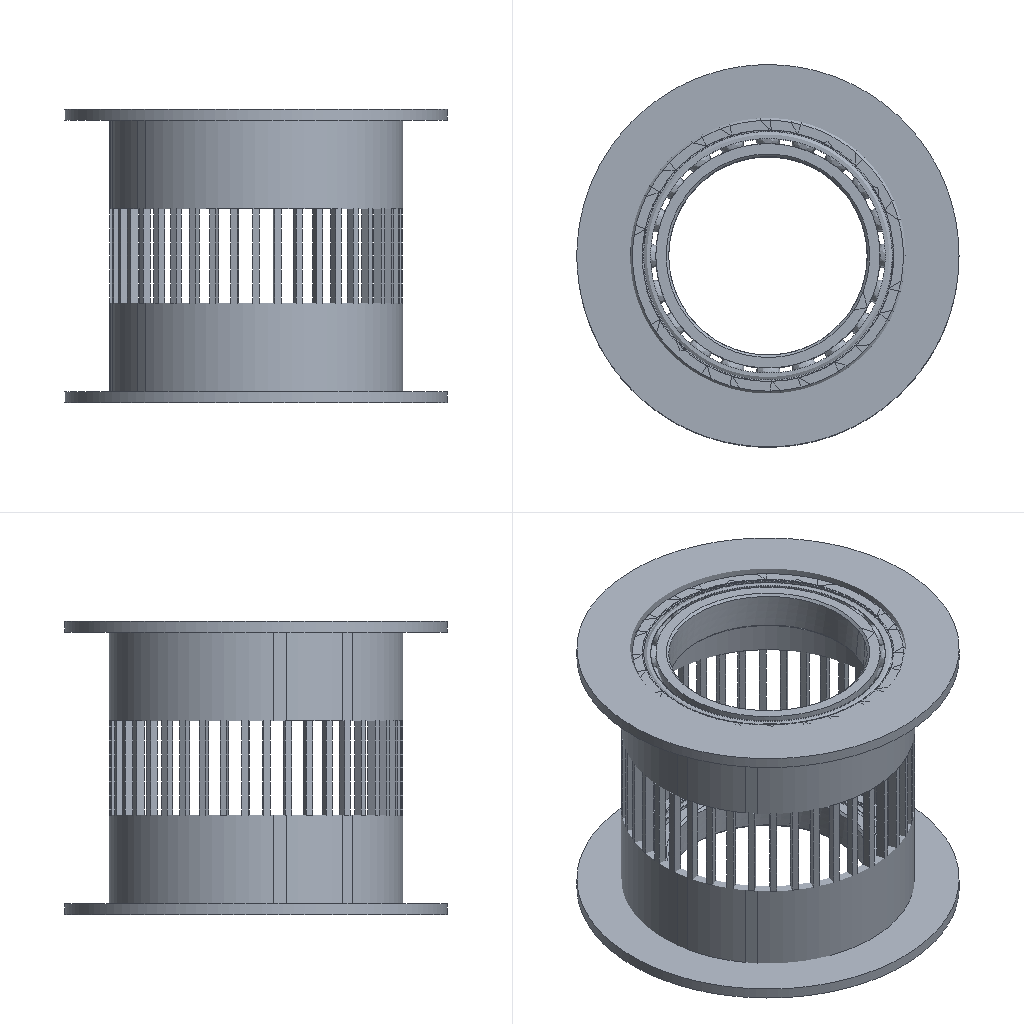Simulation study | ansys workbench
Set-up summary, first 180 of 205 lines:
category,name,step,type,value,unit,region
solver,ansys_workbench
units,SI m-kg-s (Pa),,stated,"/units,MKS"
analysis,LS1,,static
load_step,LS1,LS1,static,nsubst=1; time=1
mesh,nodes,,,153526
mesh,elements,,,97010
element_type,SOLID187,,,51778
element_type,TARGE170,,,19367
element_type,CONTA174,,,19367
element_type,SOLID186,,,5540
element_type,SURF154,,,958
material,61918_2Z|GB-T276_60000_2Z-1994,,E,2.1e+11,Pa
material,61918_2Z|GB-T276_60000_2Z-1994,,nu,0.3046
material,61918_2Z|GB-T276_60000_2Z-1994,,density,7850,kg m^-3
material,61918_2Z|GB-T276_60000_2Z-1994,,conductivity,50.44,W m^-1 C^-1
material,61918_2Z|GB-T276_60000_2Z-1994,,specific_heat,479.4,J kg^-1 C^-1
material,61918_2Z|GB-T276_60000_2Z-1994,,cte,1.196e-05,C^-1
material,"Structural Steel , S275N",,E,2.1e+11,Pa
material,"Structural Steel , S275N",,nu,0.3046
material,"Structural Steel , S275N",,density,7850,kg m^-3
material,"Structural Steel , S275N",,conductivity,50.44,W m^-1 C^-1
material,"Structural Steel , S275N",,specific_heat,479.4,J kg^-1 C^-1
material,"Structural Steel , S275N",,cte,1.196e-05,C^-1
load,Define Force Using Surface Effect Elements,LS1,surface-effect pres face 2,895386,,SURF154 #443
load,Define Force Using Surface Effect Elements,LS1,surface-effect pres face 2,895386,,SURF154 #444
load,Define Force Using Surface Effect Elements,LS1,surface-effect pres face 3,-318101,,SURF154 #445
bc,Fixed Supports,model,fixed,[dofs=ALL],,_FIXEDSU
bc,Frictionless Supports Z,model,fixed,[dofs=UZ],,_FRICSUZ
contact,Contact Region,,bonded (always),element=CONTA174
contact,Contact Region 2,,bonded (always),element=CONTA174
contact,Contact Region 3,,bonded (always),element=CONTA174
contact,Contact Region 4,,bonded (always),element=CONTA174
contact,Contact Region 5,,bonded (always),element=CONTA174
contact,Contact Region 6,,bonded (always),element=CONTA174
contact,Contact Region 7,,bonded (always),element=CONTA174
contact,Contact Region 8,,bonded (always),element=CONTA174
contact,Contact Region 9,,bonded (always),element=CONTA174
contact,Contact Region 10,,bonded (always),element=CONTA174
contact,Contact Region 11,,bonded (always),element=CONTA174
contact,Contact Region 12,,bonded (always),element=CONTA174
contact,Contact Region 13,,bonded (always),element=CONTA174
contact,Contact Region 14,,bonded (always),element=CONTA174
contact,Contact Region 15,,bonded (always),element=CONTA174
contact,Contact Region 16,,bonded (always),element=CONTA174
contact,Contact Region 17,,bonded (always),element=CONTA174
contact,Contact Region 18,,bonded (always),element=CONTA174
contact,Contact Region 19,,bonded (always),element=CONTA174
contact,Contact Region 20,,bonded (always),element=CONTA174
contact,Contact Region 21,,bonded (always),element=CONTA174
contact,Contact Region 22,,bonded (always),element=CONTA174
contact,Contact Region 23,,bonded (always),element=CONTA174
contact,Contact Region 24,,bonded (always),element=CONTA174
contact,Contact Region 25,,bonded (always),element=CONTA174
contact,Contact Region 26,,bonded (always),element=CONTA174
contact,Contact Region 27,,bonded (always),element=CONTA174
contact,Contact Region 28,,bonded (always),element=CONTA174
contact,Contact Region 29,,bonded (always),element=CONTA174
contact,Contact Region 30,,bonded (always),element=CONTA174
contact,Contact Region 31,,bonded (always),element=CONTA174
contact,Contact Region 32,,bonded (always),element=CONTA174
contact,Contact Region 33,,bonded (always),element=CONTA174
contact,Contact Region 34,,bonded (always),element=CONTA174
contact,Contact Region 35,,bonded (always),element=CONTA174
contact,Contact Region 36,,bonded (always),element=CONTA174
contact,Contact Region 37,,bonded (always),element=CONTA174
contact,Contact Region 38,,bonded (always),element=CONTA174
contact,Contact Region 39,,bonded (always),element=CONTA174
contact,Contact Region 40,,bonded (always),element=CONTA174
contact,Contact Region 41,,bonded (always),element=CONTA174
contact,Contact Region 42,,bonded (always),element=CONTA174
contact,Contact Region 43,,bonded (always),element=CONTA174
contact,Contact Region 44,,bonded (always),element=CONTA174
contact,Contact Region 45,,bonded (always),element=CONTA174
contact,Contact Region 46,,bonded (always),element=CONTA174
contact,Contact Region 47,,bonded (always),element=CONTA174
contact,Contact Region 48,,bonded (always),element=CONTA174
contact,Contact Region 49,,bonded (always),element=CONTA174
contact,Contact Region 50,,bonded (always),element=CONTA174
contact,Contact Region 51,,bonded (always),element=CONTA174
contact,Contact Region 52,,bonded (always),element=CONTA174
contact,Contact Region 53,,bonded (always),element=CONTA174
contact,Contact Region 54,,bonded (always),element=CONTA174
contact,Contact Region 55,,bonded (always),element=CONTA174
contact,Contact Region 56,,bonded (always),element=CONTA174
contact,Contact Region 57,,bonded (always),element=CONTA174
contact,Contact Region 58,,bonded (always),element=CONTA174
contact,Contact Region 59,,bonded (always),element=CONTA174
contact,Contact Region 60,,bonded (always),element=CONTA174
contact,Contact Region 61,,bonded (always),element=CONTA174
contact,Contact Region 62,,bonded (always),element=CONTA174
contact,Contact Region 63,,bonded (always),element=CONTA174
contact,Contact Region 64,,bonded (always),element=CONTA174
contact,Contact Region 65,,bonded (always),element=CONTA174
contact,Contact Region 66,,bonded (always),element=CONTA174
contact,Contact Region 67,,bonded (always),element=CONTA174
contact,Contact Region 68,,bonded (always),element=CONTA174
contact,Contact Region 69,,bonded (always),element=CONTA174
contact,Contact Region 70,,bonded (always),element=CONTA174
contact,Contact Region 71,,bonded (always),element=CONTA174
contact,Contact Region 72,,bonded (always),element=CONTA174
contact,Contact Region 73,,bonded (always),element=CONTA174
contact,Contact Region 74,,bonded (always),element=CONTA174
contact,Contact Region 75,,bonded (always),element=CONTA174
contact,Contact Region 76,,bonded (always),element=CONTA174
contact,Contact Region 77,,bonded (always),element=CONTA174
contact,Contact Region 78,,bonded (always),element=CONTA174
contact,Contact Region 79,,bonded (always),element=CONTA174
contact,Contact Region 80,,bonded (always),element=CONTA174
contact,Contact Region 81,,bonded (always),element=CONTA174
contact,Contact Region 82,,bonded (always),element=CONTA174
contact,Contact Region 83,,bonded (always),element=CONTA174
contact,Contact Region 84,,bonded (always),element=CONTA174
contact,Contact Region 85,,bonded (always),element=CONTA174
contact,Contact Region 86,,bonded (always),element=CONTA174
contact,Contact Region 87,,bonded (always),element=CONTA174
contact,Contact Region 88,,bonded (always),element=CONTA174
contact,Contact Region 89,,bonded (always),element=CONTA174
contact,Contact Region 90,,bonded (always),element=CONTA174
contact,Contact Region 91,,bonded (always),element=CONTA174
contact,Contact Region 92,,bonded (always),element=CONTA174
contact,Contact Region 93,,bonded (always),element=CONTA174
contact,Contact Region 94,,bonded (always),element=CONTA174
contact,Contact Region 95,,bonded (always),element=CONTA174
contact,Contact Region 96,,bonded (always),element=CONTA174
contact,Contact Region 97,,bonded (always),element=CONTA174
contact,Contact Region 98,,bonded (always),element=CONTA174
contact,Contact Region 99,,bonded (always),element=CONTA174
contact,Contact Region 100,,bonded (always),element=CONTA174
contact,Contact Region 101,,bonded (always),element=CONTA174
contact,Contact Region 102,,bonded (always),element=CONTA174
contact,Contact Region 103,,bonded (always),element=CONTA174
contact,Contact Region 104,,bonded (always),element=CONTA174
contact,Contact Region 105,,bonded (always),element=CONTA174
contact,Contact Region 106,,bonded (always),element=CONTA174
contact,Contact Region 107,,bonded (always),element=CONTA174
contact,Contact Region 108,,bonded (always),element=CONTA174
contact,Contact Region 109,,bonded (always),element=CONTA174
contact,Contact Region 110,,bonded (always),element=CONTA174
contact,Contact Region 111,,bonded (always),element=CONTA174
contact,Contact Region 112,,bonded (always),element=CONTA174
contact,Contact Region 113,,bonded (always),element=CONTA174
contact,Contact Region 114,,bonded (always),element=CONTA174
contact,Contact Region 115,,bonded (always),element=CONTA174
contact,Contact Region 116,,bonded (always),element=CONTA174
contact,Contact Region 117,,bonded (always),element=CONTA174
contact,Contact Region 118,,bonded (always),element=CONTA174
contact,Contact Region 119,,bonded (always),element=CONTA174
contact,Contact Region 120,,bonded (always),element=CONTA174
contact,Contact Region 121,,bonded (always),element=CONTA174
contact,Contact Region 122,,bonded (always),element=CONTA174
contact,Contact Region 123,,bonded (always),element=CONTA174
contact,Contact Region 124,,bonded (always),element=CONTA174
contact,Contact Region 125,,bonded (always),element=CONTA174
contact,Contact Region 126,,bonded (always),element=CONTA174
contact,Contact Region 127,,bonded (always),element=CONTA174
contact,Contact Region 128,,bonded (always),element=CONTA174
contact,Contact Region 129,,bonded (always),element=CONTA174
contact,Contact Region 130,,bonded (always),element=CONTA174
contact,Contact Region 131,,bonded (always),element=CONTA174
contact,Contact Region 132,,bonded (always),element=CONTA174
contact,Contact Region 133,,bonded (always),element=CONTA174
contact,Contact Region 134,,bonded (always),element=CONTA174
contact,Contact Region 135,,bonded (always),element=CONTA174
contact,Contact Region 136,,bonded (always),element=CONTA174
contact,Contact Region 137,,bonded (always),element=CONTA174
contact,Contact Region 138,,bonded (always),element=CONTA174
contact,Contact Region 139,,bonded (always),element=CONTA174
contact,Contact Region 140,,bonded (always),element=CONTA174
contact,Contact Region 141,,bonded (always),element=CONTA174
contact,Contact Region 142,,bonded (always),element=CONTA174
contact,Contact Region 143,,bonded (always),element=CONTA174
contact,Contact Region 144,,bonded (always),element=CONTA174
contact,Contact Region 145,,bonded (always),element=CONTA174
contact,Contact Region 146,,bonded (always),element=CONTA174
contact,Contact Region 147,,bonded (always),element=CONTA174
contact,Contact Region 148,,bonded (always),element=CONTA174
contact,Contact Region 149,,bonded (always),element=CONTA174
contact,Contact Region 150,,bonded (always),element=CONTA174
contact,Contact Region 151,,bonded (always),element=CONTA174
Ansys APDL input file, long lists of numbers shortened:
/batch
/config,noeldb,1     ! force off writing results to database
*get,_wallstrt,active,,time,wall
! ANSYS input file written by Workbench version 2022 R2
! File used for geometry attach:
/title,___--____ (B5)
! ****** Begin Custom Load Command Snippet ******
/COM, ACT Extensions:
/COM,     LSDYNA, 2022.2
/COM,/COM,     ANSYSMotion, 2022.2
/COM,
! ****** End   Custom Load Command Snippet ******
*DIM,_wb_ProjectScratch_dir,string,248
_wb_ProjectScratch_dir(1) = ''
*DIM,_wb_SolverFiles_dir,string,248
_wb_SolverFiles_dir(1) = ''
*DIM,_wb_userfiles_dir,string,248
_wb_userfiles_dir(1) = ''
/com,--- Data in consistent MKS units. See Solving Units in the help system for more information.
/units,MKS
/nopr
/wb,file,start              !  signify a WB generated input file
/prep7
! Turn off shape checking because checks already performed inside WB mesher.
! See help system for more information.
SHPP,OFF,,NOWARN
/nolist
etcon,set             ! allow ANSYS to choose best KEYOP's for 180x elements, resets any applicable keyopt to MAPDL defaults
/com,*********** Nodes for the whole assembly ***********
nblock,3,,168878
(1i9,3e20.9e3)
        1     5.111928775E-02    -1.660966345E-02     4.966763873E-02
! (153525 more lines like these left out)
-1
/wb,elem,start            !  set before creation of elements
/com,*********** Elements for Body 1 "GB-T276_60000_2Z-1994,61918_2Z|GB-T276_60000_2Z-1994,61918_2Z" ***********
et,1,187
eblock,19,solid,,290
(19i9)
        1        1        1        1        0        0        0        0       10        0        1        8       43       98       83      152      387      157      156
! (579 more lines like these left out)
-1
/com,*********** Elements for Body 2 "GB-T276_60000_2Z-1994,61918_2Z|GB-T276_60000_2Z-1994,61918_2Z[2]" ***********
et,2,187
eblock,19,solid,,163
(19i9)
        2        2        2        2        0        0        0        0       10        0      291      565      640      634      624      666      951      665      663
! (325 more lines like these left out)
-1
/com,*********** Elements for Body 3 "GB-T276_60000_2Z-1994,61918_2Z|GB-T276_60000_2Z-1994,61918_2Z[3]" ***********
et,3,186
keyo,3,2,1          ! set full integration on SOLID186
eblock,19,solid,,366
(19i9)
        3        3        3        3        0        0        0        0       20        0      454     1389     1537     1538     1390     1795     1474     1473     1794
! (731 more lines like these left out)
-1
/com,*********** Elements for Body 4 "GB-T276_60000_2Z-1994,61918_2Z|GB-T276_60000_2Z-1994,61918_2Z[4]" ***********
et,4,187
eblock,19,solid,,298
(19i9)
        4        4        4        4        0        0        0        0       10        0      820     3799     3885     3850     3861     3985     4248     3978     3981
! (595 more lines like these left out)
-1
/com,*********** Elements for Body 5 "GB-T276_60000_2Z-1994,61918_2Z|GB-T276_60000_2Z-1994,61918_2Z[5]" ***********
et,5,187
eblock,19,solid,,307
(19i9)
        5        5        5        5        0        0        0        0       10        0     1118     4371     4372     4394     4457     4554     4565     4557     4564
! (613 more lines like these left out)
-1
! (89 more sections like these left out)
/wb,elem,end               !  done creating elements
/com,*********** Send User Defined Coordinate System(s) ***********
csys,0
toffst,273.15,  ! Temperature offset from absolute zero
/com,*********** Set Reference Temperature ***********
tref,22.
/wb,mat,start              !  starting to send materials
/com,*********** Send Materials ***********
Temperature = 'TEMP' ! Temperature
MP,DENS,1,7850,	! kg m^-3
MP,EX,1,210000000000,	! Pa
MP,NUXY,1,0.3046,
MP,ALPX,1,1.196e-05,	! C^-1
MP,KXX,1,50.44,	! W m^-1 C^-1
MP,C,1,479.4,	! J kg^-1 C^-1
Temperature = 'TEMP' ! Temperature
MP,DENS,2,7850,	! kg m^-3
MP,EX,2,210000000000,	! Pa
MP,NUXY,2,0.3046,
MP,ALPX,2,1.196e-05,	! C^-1
MP,KXX,2,50.44,	! W m^-1 C^-1
MP,C,2,479.4,	! J kg^-1 C^-1
Temperature = 'TEMP' ! Temperature
MP,DENS,3,7850,	! kg m^-3
MP,EX,3,210000000000,	! Pa
MP,NUXY,3,0.3046,
MP,ALPX,3,1.196e-05,	! C^-1
MP,KXX,3,50.44,	! W m^-1 C^-1
MP,C,3,479.4,	! J kg^-1 C^-1
Temperature = 'TEMP' ! Temperature
MP,DENS,4,7850,	! kg m^-3
MP,EX,4,210000000000,	! Pa
MP,NUXY,4,0.3046,
MP,ALPX,4,1.196e-05,	! C^-1
MP,KXX,4,50.44,	! W m^-1 C^-1
MP,C,4,479.4,	! J kg^-1 C^-1
Temperature = 'TEMP' ! Temperature
MP,DENS,5,7850,	! kg m^-3
MP,EX,5,210000000000,	! Pa
MP,NUXY,5,0.3046,
MP,ALPX,5,1.196e-05,	! C^-1
MP,KXX,5,50.44,	! W m^-1 C^-1
MP,C,5,479.4,	! J kg^-1 C^-1
Temperature = 'TEMP' ! Temperature
MP,DENS,6,7850,	! kg m^-3
MP,EX,6,210000000000,	! Pa
MP,NUXY,6,0.3046,
MP,ALPX,6,1.196e-05,	! C^-1
MP,KXX,6,50.44,	! W m^-1 C^-1
MP,C,6,479.4,	! J kg^-1 C^-1
Temperature = 'TEMP' ! Temperature
MP,DENS,7,7850,	! kg m^-3
MP,EX,7,210000000000,	! Pa
MP,NUXY,7,0.3046,
MP,ALPX,7,1.196e-05,	! C^-1
MP,KXX,7,50.44,	! W m^-1 C^-1
MP,C,7,479.4,	! J kg^-1 C^-1
Temperature = 'TEMP' ! Temperature
MP,DENS,8,7850,	! kg m^-3
MP,EX,8,210000000000,	! Pa
MP,NUXY,8,0.3046,
MP,ALPX,8,1.196e-05,	! C^-1
MP,KXX,8,50.44,	! W m^-1 C^-1
MP,C,8,479.4,	! J kg^-1 C^-1
Temperature = 'TEMP' ! Temperature
MP,DENS,9,7850,	! kg m^-3
MP,EX,9,210000000000,	! Pa
MP,NUXY,9,0.3046,
MP,ALPX,9,1.196e-05,	! C^-1
MP,KXX,9,50.44,	! W m^-1 C^-1
MP,C,9,479.4,	! J kg^-1 C^-1
Temperature = 'TEMP' ! Temperature
MP,DENS,10,7850,	! kg m^-3
MP,EX,10,210000000000,	! Pa
MP,NUXY,10,0.3046,
MP,ALPX,10,1.196e-05,	! C^-1
MP,KXX,10,50.44,	! W m^-1 C^-1
MP,C,10,479.4,	! J kg^-1 C^-1
Temperature = 'TEMP' ! Temperature
MP,DENS,11,7850,	! kg m^-3
MP,EX,11,210000000000,	! Pa
MP,NUXY,11,0.3046,
MP,ALPX,11,1.196e-05,	! C^-1
MP,KXX,11,50.44,	! W m^-1 C^-1
MP,C,11,479.4,	! J kg^-1 C^-1
Temperature = 'TEMP' ! Temperature
MP,DENS,12,7850,	! kg m^-3
! (579 more lines like these left out)
/wb,mat,end                !  done sending materials
!************************* Model Summary ********************
!GB-T276_60000_2Z-1994,61918_2Z|GB-T276_60000_2Z-1994,61918_2Z,	结构钢，S275N,	matid,	1
!GB-T276_60000_2Z-1994,61918_2Z|GB-T276_60000_2Z-1994,61918_2Z[2],	结构钢，S275N,	matid,	2
!GB-T276_60000_2Z-1994,61918_2Z|GB-T276_60000_2Z-1994,61918_2Z[3],	结构钢，S275N,	matid,	3
! (93 more lines like these left out)
*get,_xmin,node,,mnloc,x
*get,_ymin,node,,mnloc,y
*get,_zmin,node,,mnloc,z
*get,_xmax,node,,mxloc,x
*get,_ymax,node,,mxloc,y
*get,_zmax,node,,mxloc,z
_ASMDIAG=(_xmax-_xmin)*(_xmax-_xmin)+(_ymax-_ymin)*(_ymax-_ymin)+(_zmax-_zmin)*(_zmax-_zmin)
_ASMDIAG=SQRT(_ASMDIAG)
/wb,contact,start          !  starting to send contact
/com,*********** Create Contact "接触区域" ***********
/com,            Real Constant Set For Above Contact Is 96 & 95
*set,tid,96
*set,cid,95
r,tid
r,cid
et,tid,170
et,cid,174
eblock,10,,,86
(15i9)
   108555       96       96       96        0       55       58       28       28      435      314       28      312
! (85 more lines like these left out)
-1
eblock,10,,,86
(15i9)
   108641       95       95       95        0       55       58       28       28      435      314       28      312
! (85 more lines like these left out)
-1
eblock,10,,,15
(15i9)
   108727       95       96       95        0     1615     1616     1136     1135     3538     2274     2267     2269
! (14 more lines like these left out)
-1
eblock,10,,,15
(15i9)
   108742       96       95       96        0     1615     1616     1136     1135     3538     2274     2267     2269
! (14 more lines like these left out)
-1
keyo,cid,8,2               ! auto create asymmetric contact (from Program Controlled setting)
keyo,cid,10,0              ! adjust contact stiffness each NR iteration (from Program Controlled setting)
keyo,cid,12,5              ! bonded always
keyo,cid,18,1              ! small sliding turned on by application
keyo,cid,2,0               ! augmented Lagrange (from Program Controlled setting)
keyo,cid,4,0               ! on Gauss point (from Program Controlled setting)
keyo,cid,9,1               ! ignore initial gaps/penetration
keyo,cid,7,0               ! No Prediction
rmod,tid,3,10.      ! FKN
rmod,tid,5,0.       ! ICONT
rmod,tid,6,0.       ! PINB
rmod,tid,10,0.      ! CNOF
rmod,tid,12,0.      ! FKT
rmod,tid,36,305     ! WB DSID
rmod,cid,3,10.      ! FKN
rmod,cid,5,0.       ! ICONT
rmod,cid,6,0.       ! PINB
rmod,cid,10,0.      ! CNOF
rmod,cid,12,0.      ! FKT
rmod,cid,36,305     ! WB DSID
/com,*********** Create Contact "接触区域 2" ***********
/com,            Real Constant Set For Above Contact Is 98 & 97
*set,tid,98
*set,cid,97
r,tid
r,cid
et,tid,170
et,cid,174
eblock,10,,,91
(15i9)
   108757       98       98       98        0       19       39       41       41      243      368       41      244
! (90 more lines like these left out)
-1
eblock,10,,,91
(15i9)
   108848       97       97       97        0       19       39       41       41      243      368       41      244
! (90 more lines like these left out)
-1
eblock,10,,,15
(15i9)
   108939       97       98       97        0    60122    60123    60039    60038    63262    63098    63095    63096
! (14 more lines like these left out)
-1
eblock,10,,,15
(15i9)
   108954       98       97       98        0    60122    60123    60039    60038    63262    63098    63095    63096
! (14 more lines like these left out)
-1
keyo,cid,8,2               ! auto create asymmetric contact (from Program Controlled setting)
keyo,cid,10,0              ! adjust contact stiffness each NR iteration (from Program Controlled setting)
keyo,cid,12,5              ! bonded always
keyo,cid,18,1              ! small sliding turned on by application
keyo,cid,2,0               ! augmented Lagrange (from Program Controlled setting)
keyo,cid,4,0               ! on Gauss point (from Program Controlled setting)
keyo,cid,9,1               ! ignore initial gaps/penetration
keyo,cid,7,0               ! No Prediction
rmod,tid,3,10.      ! FKN
rmod,tid,5,0.       ! ICONT
rmod,tid,6,0.       ! PINB
rmod,tid,10,0.      ! CNOF
rmod,tid,12,0.      ! FKT
rmod,tid,36,308     ! WB DSID
rmod,cid,3,10.      ! FKN
rmod,cid,5,0.       ! ICONT
rmod,cid,6,0.       ! PINB
rmod,cid,10,0.      ! CNOF
rmod,cid,12,0.      ! FKT
rmod,cid,36,308     ! WB DSID
/com,*********** Create Contact "接触区域 3" ***********
/com,            Real Constant Set For Above Contact Is 100 & 99
*set,tid,100
*set,cid,99
r,tid
r,cid
et,tid,170
et,cid,174
eblock,10,,,94
(15i9)
   108969      100      100      100        0      616      619      589      589      914      821      589      819
! (93 more lines like these left out)
-1
eblock,10,,,94
(15i9)
   109063       99       99       99        0      616      619      589      589      914      821      589      819
! (93 more lines like these left out)
-1
eblock,10,,,13
(15i9)
   109157       99      100       99        0     1612     1613     1133     1132     3532     2263     2258     2260
! (12 more lines like these left out)
-1
eblock,10,,,13
(15i9)
   109170      100       99      100        0     1612     1613     1133     1132     3532     2263     2258     2260
! (12 more lines like these left out)
-1
keyo,cid,8,2               ! auto create asymmetric contact (from Program Controlled setting)
keyo,cid,10,0              ! adjust contact stiffness each NR iteration (from Program Controlled setting)
keyo,cid,12,5              ! bonded always
keyo,cid,18,1              ! small sliding turned on by application
keyo,cid,2,0               ! augmented Lagrange (from Program Controlled setting)
keyo,cid,4,0               ! on Gauss point (from Program Controlled setting)
keyo,cid,9,1               ! ignore initial gaps/penetration
keyo,cid,7,0               ! No Prediction
rmod,tid,3,10.      ! FKN
rmod,tid,5,0.       ! ICONT
rmod,tid,6,0.       ! PINB
rmod,tid,10,0.      ! CNOF
rmod,tid,12,0.      ! FKT
rmod,tid,36,311     ! WB DSID
rmod,cid,3,10.      ! FKN
rmod,cid,5,0.       ! ICONT
rmod,cid,6,0.       ! PINB
rmod,cid,10,0.      ! CNOF
rmod,cid,12,0.      ! FKT
rmod,cid,36,311     ! WB DSID
/com,*********** Create Contact "接触区域 4" ***********
/com,            Real Constant Set For Above Contact Is 102 & 101
*set,tid,102
*set,cid,101
r,tid
r,cid
et,tid,170
et,cid,174
eblock,10,,,97
(15i9)
   109183      102      102      102        0      616      619      589      589      914      821      589      819
! (96 more lines like these left out)
-1
eblock,10,,,97
(15i9)
   109280      101      101      101        0      616      619      589      589      914      821      589      819
! (96 more lines like these left out)
-1
eblock,10,,,13
(15i9)
   109377      101      102      101        0    60119    60120    60036    60035    63256    63092    63089    63090
! (12 more lines like these left out)
-1
eblock,10,,,13
(15i9)
   109390      102      101      102        0    60119    60120    60036    60035    63256    63092    63089    63090
! (12 more lines like these left out)
-1
keyo,cid,8,2               ! auto create asymmetric contact (from Program Controlled setting)
keyo,cid,10,0              ! adjust contact stiffness each NR iteration (from Program Controlled setting)
keyo,cid,12,5              ! bonded always
keyo,cid,18,1              ! small sliding turned on by application
keyo,cid,2,0               ! augmented Lagrange (from Program Controlled setting)
keyo,cid,4,0               ! on Gauss point (from Program Controlled setting)
keyo,cid,9,1               ! ignore initial gaps/penetration
keyo,cid,7,0               ! No Prediction
rmod,tid,3,10.      ! FKN
rmod,tid,5,0.       ! ICONT
rmod,tid,6,0.       ! PINB
rmod,tid,10,0.      ! CNOF
rmod,tid,12,0.      ! FKT
rmod,tid,36,314     ! WB DSID
rmod,cid,3,10.      ! FKN
rmod,cid,5,0.       ! ICONT
rmod,cid,6,0.       ! PINB
rmod,cid,10,0.      ! CNOF
rmod,cid,12,0.      ! FKT
rmod,cid,36,314     ! WB DSID
/com,*********** Create Contact "接触区域 5" ***********
/com,            Real Constant Set For Above Contact Is 104 & 103
*set,tid,104
*set,cid,103
r,tid
r,cid
et,tid,170
et,cid,174
eblock,10,,,14
(15i9)
   109403      104      104      104        0     1562     1563     1083     1082     3431     2113     2108     2110
! (13 more lines like these left out)
-1
eblock,10,,,14
(15i9)
   109417      103      103      103        0     1562     1563     1083     1082     3431     2113     2108     2110
! (13 more lines like these left out)
-1
eblock,10,,,86
(15i9)
   109431      103      104      103        0     3841     3844     3814     3814     4213     4091     3814     4089
! (85 more lines like these left out)
-1
eblock,10,,,86
(15i9)
   109517      104      103      104        0     3841     3844     3814     3814     4213     4091     3814     4089
! (85 more lines like these left out)
-1
keyo,cid,8,2               ! auto create asymmetric contact (from Program Controlled setting)
keyo,cid,10,0              ! adjust contact stiffness each NR iteration (from Program Controlled setting)
keyo,cid,12,5              ! bonded always
keyo,cid,18,1              ! small sliding turned on by application
keyo,cid,2,0               ! augmented Lagrange (from Program Controlled setting)
keyo,cid,4,0               ! on Gauss point (from Program Controlled setting)
keyo,cid,9,1               ! ignore initial gaps/penetration
keyo,cid,7,0               ! No Prediction
rmod,tid,3,10.      ! FKN
rmod,tid,5,0.       ! ICONT
rmod,tid,6,0.       ! PINB
rmod,tid,10,0.      ! CNOF
rmod,tid,12,0.      ! FKT
rmod,tid,36,317     ! WB DSID
rmod,cid,3,10.      ! FKN
rmod,cid,5,0.       ! ICONT
rmod,cid,6,0.       ! PINB
rmod,cid,10,0.      ! CNOF
rmod,cid,12,0.      ! FKT
rmod,cid,36,317     ! WB DSID
! (169 more sections like these left out)
/wb,contact,end            !  done creating contacts
/golist
/wb,load,start             !  starting to send loads
/com,*********** Fixed Supports ***********
CMBLOCK,_FIXEDSU,NODE,     1806
(8i10)
    128434    128435    128436    128437    128438    128439    128440    128441
! (225 more lines like these left out)
cmsel,s,_FIXEDSU
d,all,all
nsel,all
/com,********* Frictionless Supports Z *********
CMBLOCK,_FRICSUZ,NODE,     7092
(8i10)
      1139      1140      1141      1142      1143      1144      1145      1146
! (886 more lines like these left out)
cmsel,s,_FRICSUZ
d,all,uz,0
nsel,all
/com,*********** Node Rotations ***********
nmod,1213,,,,-90.,0.,180.
nmod,1321,,,,0.,0.,-180.
nmod,1322,,,,0.,0.,-180.
nmod,1323,,,,0.,0.,-180.
! (116 more lines like these left out)
/com,*********** Define Force Using Surface Effect Elements ***********
local,12,0,0.,0.,0.,0.,0.,0.
csys,0
et,443,154
eblock,10,,,244
(15i9)
   147289      443      443      443       12     1259     1322     1321     1319     2704     2889     2883     2703
! (243 more lines like these left out)
-1
esel,s,type,,443
keyop,443,2,1                ! Apply load in local coordinate system
keyop,443,7,1                ! Use original area so load is constant in large deformation
esel,all
/com,*********** Define Force Using Surface Effect Elements ***********
local,13,0,0.,0.,0.,0.,0.,0.
csys,0
et,444,154
eblock,10,,,244
(15i9)
   147533      444      444      444       13    65471    65534    65533    65531    66916    67101    67095    66915
! (243 more lines like these left out)
-1
esel,s,type,,444
keyop,444,2,1                ! Apply load in local coordinate system
keyop,444,7,1                ! Use original area so load is constant in large deformation
esel,all
/com,*********** Define Force Using Surface Effect Elements ***********
local,14,0,0.,0.,0.,0.,0.,0.
csys,0
et,445,154
eblock,10,,,470
(15i9)
   147777      445      445      445       14   140329   140275   140327   140328   144099   144098   144182   144183
! (469 more lines like these left out)
-1
esel,s,type,,445
keyop,445,2,1                ! Apply load in local coordinate system
keyop,445,7,1                ! Use original area so load is constant in large deformation
esel,all
/gst,on,on
fini
*get,_numnode,node,0,count
*get,_numelem,elem,0,count
*get, _MAXELEMNUM, elem, 0, NUM, MAX
*get, _MAXNODENUM, node, 0, NUM, MAX
*get, _MAXELEMTYPE, etyp, 0, NUM, MAX
*get, _MAXREALCONST, rcon, 0, NUM, MAX
/go
/wb,load,end               !  done creating loads
/com,--- Number of total nodes = %_numnode%
/com,--- Number of contact elements = 39692
/com,--- Number of spring elements = 0
/com,--- Number of bearing elements = 0
/com,--- Number of solid elements = 57318
/com,--- Number of condensed parts = 0
/com,--- Number of total elements = %_numelem%
*get,_wallbsol,active,,time,wall
/com,****************************************************************************
/com,*************************    SOLUTION       ********************************
/com,****************************************************************************
/solu
antype,0                   ! static analysis
_thickRatio=0.319   ! Ratio of thick parts in the model
eqsl,sparse,,,,,1
cntr,print,1               ! print out contact info and also make no initial contact an error
cntr,out,yes               ! write contact output to file.cmn due to many contact pairs present
dmpoption,emat,no             ! Don't combine emat file for DANSYS
dmpoption,esav,no             ! Don't combine esav file for DANSYS
nldiag,cont,iter           ! print out contact info each equilibrium iteration
rescontrol,,none                 ! Do not keep any restart files
/com,****************************************************
/com,******************* SOLVE FOR LS 1 OF 1 ****************
esel,s,type,,443
nsle
sfe,all,1,pres,1,0.
sfe,all,2,pres,1,895386.369
sfe,all,3,pres,1,0.
esel,s,type,,444
nsle
sfe,all,1,pres,1,0.
sfe,all,2,pres,1,895386.369
sfe,all,3,pres,1,0.
esel,s,type,,445
nsle
sfe,all,1,pres,1,0.
sfe,all,2,pres,1,0.
sfe,all,3,pres,1,-318101.19
nsel,all
esel,all
/nopr
/gopr
nsub,1,1,1
time,1.
outres,erase
outres,all,none
outres,nsol,all,
outres,rsol,all
outres,eangl,all
outres,etmp,all
outres,veng,all
outres,strs,all,
outres,epel,all,
outres,eppl,all,
outres,cont,all,
! *********** WB SOLVE COMMAND ***********
! check interactive state
*get,ANSINTER_,active,,int
*if,ANSINTER_,ne,0,then
/eof
*endif
solve
/com *************** Write FE CONNECTORS *********
CEWRITE,file,ce,,INTE
/com,****************************************************
/com,*************** FINISHED SOLVE FOR LS 1 *************
*get,_wallasol,active,,time,wall
/nopr
*get,_numnode,node,0,count
*get,_numelem,elem,0,count
*get, _MAXELEMNUM, elem, 0, NUM, MAX
*get, _MAXNODENUM, node, 0, NUM, MAX,,,INTERNAL
*get, _MAXELEMTYPE, etyp, 0, NUM, MAX
*get, _MAXREALCONST, rcon, 0, NUM, MAX
*get,_NSOLTHREADS,active,0,ntfs
*get,_NSOLPROCESSES,active,0,npfs
/gopr
/post1
xmlo,ENCODING,ISO-8859-1
xmlo,parm
/xml,parm,xml
fini
/gopr
*get,_walldone,active,,time,wall
_preptime=(_wallbsol-_wallstrt)*3600
_solvtime=(_wallasol-_wallbsol)*3600
_posttime=(_walldone-_wallasol)*3600
_totaltim=(_walldone-_wallstrt)*3600
*get,_dlbratio,active,0,solu,dlbr
*get,_combtime,active,0,solu,comb
*get,_ssmode,active,0,solu,ssmm
*get,_ndofs,active,0,solu,ndof
*get,_sol_end_time,active,0,set,time
*if,_sol_end_time,eq,1.,then
/fclean				!clean distributed files
*endif
/com,--- Total number of nodes = %_numnode%
/com,--- Total number of elements = %_numelem%
/com,--- Element load balance ratio = %_dlbratio%
/com,--- Time to combine distributed files = %_combtime%
/com,--- Sparse memory mode = %_ssmode%
/com,--- Number of DOF = %_ndofs%
/wb,file,end               ! done with WB generated input
Results summary:
result,analyses[0].index,,,1
result,analyses[0].system,,,SYS
result,analyses[0].deck,,,deck.dat
result,analyses[0].solve_status,,,completed
result,analyses[0].analysis_type,,,static
result,analyses[0].physics,,,mechanical
result,analyses[0].unit_system,,,"MKS: m, kg, N, s, V, A, degC"
result,analyses[0].n_sets,,,1
result,analyses[0].load_steps[0].set,set=1,,1
result,analyses[0].load_steps[0].time_or_freq,set=1,,1
result,analyses[0].load_steps[0].max_displacement_magnitude,set=1,,3.20357e-06
result,analyses[0].load_steps[0].max_von_mises_nodal,set=1,,3.95767e+07
result,analyses[0].load_steps[0].reaction_force_sum_xyz[1],set=1,,-1.2864e-07
result,analyses[0].load_steps[0].reaction_force_sum_xyz[2],set=1,,-8000
result,analyses[0].load_steps[0].reaction_force_sum_xyz[3],set=1,,3600